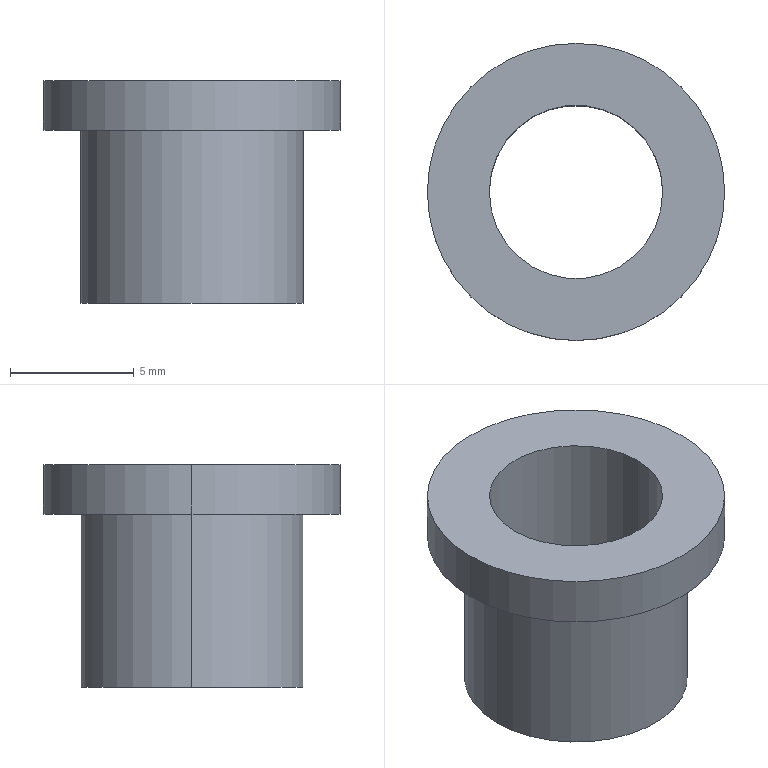Part | SolidWorks | features Extrusion 1, ICE 1 | 1 solid | 9 faces | box 12 x 12 x 9 mm | volume 325.155 mm3 | cylinder 6 | plane 3 | commonest cylinder face diameters 7 x2 9 x2 12 x2
STEP:
#1=CARTESIAN_POINT('',(4.5,0.,-8.));
#2=VERTEX_POINT('',#1);
#3=CARTESIAN_POINT('',(-4.5,0.,-8.));
#4=VERTEX_POINT('',#3);
#5=CARTESIAN_POINT('',(0.,0.,-8.));
#6=DIRECTION('',(0.,0.,1.));
#7=DIRECTION('',(1.,0.,0.));
#8=AXIS2_PLACEMENT_3D('',#5,#6,#7);
#9=CIRCLE('',#8,4.5);
#10=EDGE_CURVE('',#2,#4,#9,.T.);
#11=ORIENTED_EDGE('',*,*,#10,.T.);
#12=CARTESIAN_POINT('',(-4.5,0.,-1.));
#13=VERTEX_POINT('',#12);
#14=CARTESIAN_POINT('',(-4.5,0.,-8.));
#15=DIRECTION('',(0.,0.,1.));
#16=VECTOR('',#15,1000.);
#17=LINE('',#14,#16);
#18=EDGE_CURVE('',#4,#13,#17,.T.);
#19=ORIENTED_EDGE('',*,*,#18,.T.);
#20=CARTESIAN_POINT('',(4.5,0.,-1.));
#21=VERTEX_POINT('',#20);
#22=CARTESIAN_POINT('',(0.,0.,-1.));
#23=DIRECTION('',(0.,0.,1.));
#24=DIRECTION('',(1.,0.,0.));
#25=AXIS2_PLACEMENT_3D('',#22,#23,#24);
#26=CIRCLE('',#25,4.5);
#27=EDGE_CURVE('',#21,#13,#26,.T.);
#28=ORIENTED_EDGE('',*,*,#27,.F.);
#29=CARTESIAN_POINT('',(4.5,0.,-8.));
#30=DIRECTION('',(0.,0.,1.));
#31=VECTOR('',#30,1000.);
#32=LINE('',#29,#31);
#33=EDGE_CURVE('',#2,#21,#32,.T.);
#34=ORIENTED_EDGE('',*,*,#33,.F.);
#35=EDGE_LOOP('',(#11,#19,#28,#34));
#36=FACE_OUTER_BOUND('',#35,.T.);
#37=CARTESIAN_POINT('',(0.,0.,-8.));
#38=DIRECTION('',(0.,0.,1.));
#39=DIRECTION('',(1.,0.,0.));
#40=AXIS2_PLACEMENT_3D('',#37,#38,#39);
#41=CYLINDRICAL_SURFACE('',#40,4.5);
#42=ADVANCED_FACE('',(#36),#41,.T.);
#43=CARTESIAN_POINT('',(-3.5,0.,-8.));
#44=VERTEX_POINT('',#43);
#45=CARTESIAN_POINT('',(3.5,0.,-8.));
#46=VERTEX_POINT('',#45);
#47=CARTESIAN_POINT('',(0.,0.,-8.));
#48=DIRECTION('',(0.,0.,1.));
#49=DIRECTION('',(1.,0.,0.));
#50=AXIS2_PLACEMENT_3D('',#47,#48,#49);
#51=CIRCLE('',#50,3.5);
#52=EDGE_CURVE('',#44,#46,#51,.T.);
#53=ORIENTED_EDGE('',*,*,#52,.F.);
#54=CARTESIAN_POINT('',(-3.5,0.,1.));
#55=VERTEX_POINT('',#54);
#56=CARTESIAN_POINT('',(-3.5,0.,-1.));
#57=DIRECTION('',(0.,0.,1.));
#58=VECTOR('',#57,1000.);
#59=LINE('',#56,#58);
#60=EDGE_CURVE('',#44,#55,#59,.T.);
#61=ORIENTED_EDGE('',*,*,#60,.T.);
#62=CARTESIAN_POINT('',(3.5,0.,1.));
#63=VERTEX_POINT('',#62);
#64=CARTESIAN_POINT('',(0.,0.,1.));
#65=DIRECTION('',(0.,0.,1.));
#66=DIRECTION('',(1.,0.,0.));
#67=AXIS2_PLACEMENT_3D('',#64,#65,#66);
#68=CIRCLE('',#67,3.5);
#69=EDGE_CURVE('',#55,#63,#68,.T.);
#70=ORIENTED_EDGE('',*,*,#69,.T.);
#71=CARTESIAN_POINT('',(3.5,0.,-1.));
#72=DIRECTION('',(0.,0.,1.));
#73=VECTOR('',#72,1000.);
#74=LINE('',#71,#73);
#75=EDGE_CURVE('',#46,#63,#74,.T.);
#76=ORIENTED_EDGE('',*,*,#75,.F.);
#77=EDGE_LOOP('',(#53,#61,#70,#76));
#78=FACE_OUTER_BOUND('',#77,.T.);
#79=CARTESIAN_POINT('',(0.,0.,-1.));
#80=DIRECTION('',(0.,0.,1.));
#81=DIRECTION('',(1.,0.,0.));
#82=AXIS2_PLACEMENT_3D('',#79,#80,#81);
#83=CYLINDRICAL_SURFACE('',#82,3.5);
#84=ADVANCED_FACE('',(#78),#83,.F.);
#85=CARTESIAN_POINT('',(6.,0.,-1.));
#86=VERTEX_POINT('',#85);
#87=CARTESIAN_POINT('',(-6.,0.,-1.));
#88=VERTEX_POINT('',#87);
#89=CARTESIAN_POINT('',(0.,0.,-1.));
#90=DIRECTION('',(0.,0.,1.));
#91=DIRECTION('',(1.,0.,0.));
#92=AXIS2_PLACEMENT_3D('',#89,#90,#91);
#93=CIRCLE('',#92,6.);
#94=EDGE_CURVE('',#86,#88,#93,.T.);
#95=ORIENTED_EDGE('',*,*,#94,.T.);
#96=CARTESIAN_POINT('',(-6.,0.,1.));
#97=VERTEX_POINT('',#96);
#98=CARTESIAN_POINT('',(-6.,0.,-1.));
#99=DIRECTION('',(0.,0.,1.));
#100=VECTOR('',#99,1000.);
#101=LINE('',#98,#100);
#102=EDGE_CURVE('',#88,#97,#101,.T.);
#103=ORIENTED_EDGE('',*,*,#102,.T.);
#104=CARTESIAN_POINT('',(6.,0.,1.));
#105=VERTEX_POINT('',#104);
#106=CARTESIAN_POINT('',(0.,0.,1.));
#107=DIRECTION('',(0.,0.,1.));
#108=DIRECTION('',(1.,0.,0.));
#109=AXIS2_PLACEMENT_3D('',#106,#107,#108);
#110=CIRCLE('',#109,6.);
#111=EDGE_CURVE('',#105,#97,#110,.T.);
#112=ORIENTED_EDGE('',*,*,#111,.F.);
#113=CARTESIAN_POINT('',(6.,0.,-1.));
#114=DIRECTION('',(0.,0.,1.));
#115=VECTOR('',#114,1000.);
#116=LINE('',#113,#115);
#117=EDGE_CURVE('',#86,#105,#116,.T.);
#118=ORIENTED_EDGE('',*,*,#117,.F.);
#119=EDGE_LOOP('',(#95,#103,#112,#118));
#120=FACE_OUTER_BOUND('',#119,.T.);
#121=CARTESIAN_POINT('',(0.,0.,-1.));
#122=DIRECTION('',(0.,0.,1.));
#123=DIRECTION('',(1.,0.,0.));
#124=AXIS2_PLACEMENT_3D('',#121,#122,#123);
#125=CYLINDRICAL_SURFACE('',#124,6.);
#126=ADVANCED_FACE('',(#120),#125,.T.);
#127=ORIENTED_EDGE('',*,*,#102,.F.);
#128=CARTESIAN_POINT('',(0.,0.,-1.));
#129=DIRECTION('',(0.,0.,1.));
#130=DIRECTION('',(1.,0.,0.));
#131=AXIS2_PLACEMENT_3D('',#128,#129,#130);
#132=CIRCLE('',#131,6.);
#133=EDGE_CURVE('',#88,#86,#132,.T.);
#134=ORIENTED_EDGE('',*,*,#133,.T.);
#135=ORIENTED_EDGE('',*,*,#117,.T.);
#136=CARTESIAN_POINT('',(0.,0.,1.));
#137=DIRECTION('',(0.,0.,1.));
#138=DIRECTION('',(1.,0.,0.));
#139=AXIS2_PLACEMENT_3D('',#136,#137,#138);
#140=CIRCLE('',#139,6.);
#141=EDGE_CURVE('',#97,#105,#140,.T.);
#142=ORIENTED_EDGE('',*,*,#141,.F.);
#143=EDGE_LOOP('',(#127,#134,#135,#142));
#144=FACE_OUTER_BOUND('',#143,.T.);
#145=CARTESIAN_POINT('',(0.,0.,-1.));
#146=DIRECTION('',(0.,0.,1.));
#147=DIRECTION('',(1.,0.,0.));
#148=AXIS2_PLACEMENT_3D('',#145,#146,#147);
#149=CYLINDRICAL_SURFACE('',#148,6.);
#150=ADVANCED_FACE('',(#144),#149,.T.);
#151=ORIENTED_EDGE('',*,*,#27,.T.);
#152=CARTESIAN_POINT('',(0.,0.,-1.));
#153=DIRECTION('',(0.,0.,1.));
#154=DIRECTION('',(1.,0.,0.));
#155=AXIS2_PLACEMENT_3D('',#152,#153,#154);
#156=CIRCLE('',#155,4.5);
#157=EDGE_CURVE('',#13,#21,#156,.T.);
#158=ORIENTED_EDGE('',*,*,#157,.T.);
#159=EDGE_LOOP('',(#151,#158));
#160=FACE_BOUND('',#159,.T.);
#161=ORIENTED_EDGE('',*,*,#94,.F.);
#162=ORIENTED_EDGE('',*,*,#133,.F.);
#163=EDGE_LOOP('',(#161,#162));
#164=FACE_OUTER_BOUND('',#163,.T.);
#165=CARTESIAN_POINT('',(0.,0.,-1.));
#166=DIRECTION('',(0.,0.,1.));
#167=DIRECTION('',(1.,0.,0.));
#168=AXIS2_PLACEMENT_3D('',#165,#166,#167);
#169=PLANE('',#168);
#170=ADVANCED_FACE('',(#160,#164),#169,.F.);
#171=CARTESIAN_POINT('',(0.,0.,1.));
#172=DIRECTION('',(0.,0.,1.));
#173=DIRECTION('',(1.,0.,0.));
#174=AXIS2_PLACEMENT_3D('',#171,#172,#173);
#175=CIRCLE('',#174,3.5);
#176=EDGE_CURVE('',#63,#55,#175,.T.);
#177=ORIENTED_EDGE('',*,*,#176,.F.);
#178=ORIENTED_EDGE('',*,*,#69,.F.);
#179=EDGE_LOOP('',(#177,#178));
#180=FACE_BOUND('',#179,.T.);
#181=ORIENTED_EDGE('',*,*,#111,.T.);
#182=ORIENTED_EDGE('',*,*,#141,.T.);
#183=EDGE_LOOP('',(#181,#182));
#184=FACE_OUTER_BOUND('',#183,.T.);
#185=CARTESIAN_POINT('',(0.,0.,1.));
#186=DIRECTION('',(0.,0.,1.));
#187=DIRECTION('',(1.,0.,0.));
#188=AXIS2_PLACEMENT_3D('',#185,#186,#187);
#189=PLANE('',#188);
#190=ADVANCED_FACE('',(#180,#184),#189,.T.);
#191=ORIENTED_EDGE('',*,*,#60,.F.);
#192=CARTESIAN_POINT('',(0.,0.,-8.));
#193=DIRECTION('',(0.,0.,1.));
#194=DIRECTION('',(1.,0.,0.));
#195=AXIS2_PLACEMENT_3D('',#192,#193,#194);
#196=CIRCLE('',#195,3.5);
#197=EDGE_CURVE('',#46,#44,#196,.T.);
#198=ORIENTED_EDGE('',*,*,#197,.F.);
#199=ORIENTED_EDGE('',*,*,#75,.T.);
#200=ORIENTED_EDGE('',*,*,#176,.T.);
#201=EDGE_LOOP('',(#191,#198,#199,#200));
#202=FACE_OUTER_BOUND('',#201,.T.);
#203=CARTESIAN_POINT('',(0.,0.,-1.));
#204=DIRECTION('',(0.,0.,1.));
#205=DIRECTION('',(1.,0.,0.));
#206=AXIS2_PLACEMENT_3D('',#203,#204,#205);
#207=CYLINDRICAL_SURFACE('',#206,3.5);
#208=ADVANCED_FACE('',(#202),#207,.F.);
#209=ORIENTED_EDGE('',*,*,#18,.F.);
#210=CARTESIAN_POINT('',(0.,0.,-8.));
#211=DIRECTION('',(0.,0.,1.));
#212=DIRECTION('',(1.,0.,0.));
#213=AXIS2_PLACEMENT_3D('',#210,#211,#212);
#214=CIRCLE('',#213,4.5);
#215=EDGE_CURVE('',#4,#2,#214,.T.);
#216=ORIENTED_EDGE('',*,*,#215,.T.);
#217=ORIENTED_EDGE('',*,*,#33,.T.);
#218=ORIENTED_EDGE('',*,*,#157,.F.);
#219=EDGE_LOOP('',(#209,#216,#217,#218));
#220=FACE_OUTER_BOUND('',#219,.T.);
#221=CARTESIAN_POINT('',(0.,0.,-8.));
#222=DIRECTION('',(0.,0.,1.));
#223=DIRECTION('',(1.,0.,0.));
#224=AXIS2_PLACEMENT_3D('',#221,#222,#223);
#225=CYLINDRICAL_SURFACE('',#224,4.5);
#226=ADVANCED_FACE('',(#220),#225,.T.);
#227=ORIENTED_EDGE('',*,*,#197,.T.);
#228=ORIENTED_EDGE('',*,*,#52,.T.);
#229=EDGE_LOOP('',(#227,#228));
#230=FACE_BOUND('',#229,.T.);
#231=ORIENTED_EDGE('',*,*,#10,.F.);
#232=ORIENTED_EDGE('',*,*,#215,.F.);
#233=EDGE_LOOP('',(#231,#232));
#234=FACE_OUTER_BOUND('',#233,.T.);
#235=CARTESIAN_POINT('',(0.,0.,-8.));
#236=DIRECTION('',(0.,0.,1.));
#237=DIRECTION('',(1.,0.,0.));
#238=AXIS2_PLACEMENT_3D('',#235,#236,#237);
#239=PLANE('',#238);
#240=ADVANCED_FACE('',(#230,#234),#239,.F.);
#241=CLOSED_SHELL('',(#42,#84,#126,#150,#170,#190,#208,#226,#240));
#242=MANIFOLD_SOLID_BREP('',#241);
#243=CARTESIAN_POINT('',(0.,0.,0.));
#244=DIRECTION('',(0.,0.,1.));
#245=DIRECTION('',(1.,0.,0.));
#246=AXIS2_PLACEMENT_3D('',#243,#244,#245);
#247=(LENGTH_UNIT()NAMED_UNIT(*)SI_UNIT(.MILLI.,.METRE.));
#248=UNCERTAINTY_MEASURE_WITH_UNIT(LENGTH_MEASURE(0.00001),#247,'','');
#249=(NAMED_UNIT(*)PLANE_ANGLE_UNIT()SI_UNIT($,.RADIAN.));
#250=(NAMED_UNIT(*)SI_UNIT($,.STERADIAN.)SOLID_ANGLE_UNIT());
#251=(GEOMETRIC_REPRESENTATION_CONTEXT(3)GLOBAL_UNCERTAINTY_ASSIGNED_CONTEXT((#248))GLOBAL_UNIT_ASSIGNED_CONTEXT((#247,#249,#250))REPRESENTATION_CONTEXT('',''));
#252=ADVANCED_BREP_SHAPE_REPRESENTATION('',(#242,#246),#251);